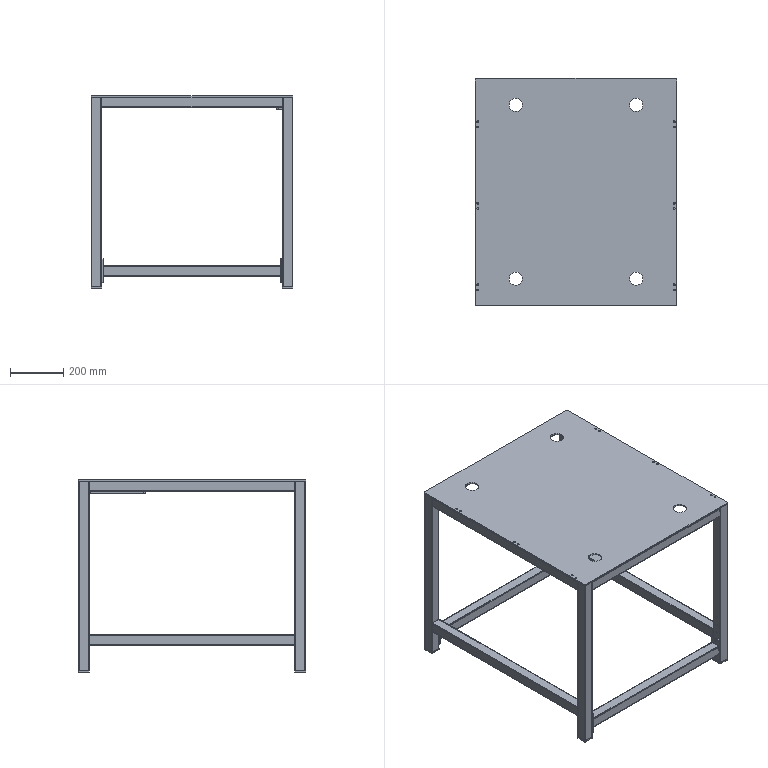Part | SolidWorks | features ICE 14, Fillet 3, Cut 1, Extrusion 1, LPattern 1 | 22 solids | 493 faces | box 755 x 850 x 720 mm | volume 5913243 mm3 | cylinder 295 | plane 198 | commonest cylinder face diameters 6 x68 5 x60 6.8 x60 2 x48 8 x24 10 x19